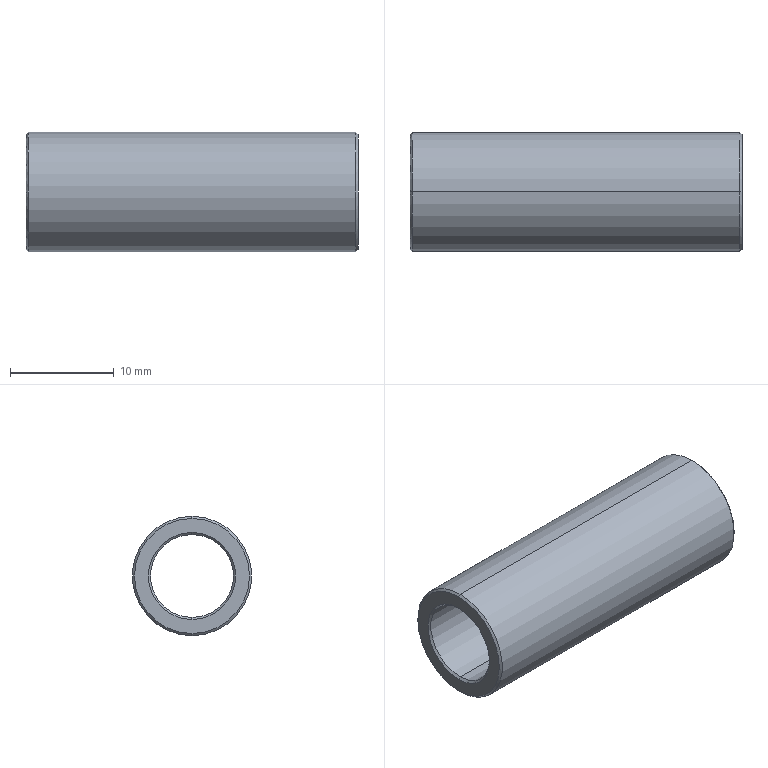Part | STEP file | FNCLSS-V8-D11.5-L32.0 | 1 solid | 14 faces | box 32 x 11.5 x 11.5 mm | volume 1713 mm3 | cone 8 | cylinder 4 | plane 2 | commonest cylinder face diameters 8 x2 11.5 x2
STEP:
#1=CARTESIAN_POINT('',(0.,0.,0.));
#2=DIRECTION('',(0.,0.,1.));
#3=DIRECTION('',(1.,0.,0.));
#4=AXIS2_PLACEMENT_3D('',#1,#2,#3);
#5=CARTESIAN_POINT('',(32.,0.,-5.55));
#6=VERTEX_POINT('',#5);
#7=CARTESIAN_POINT('',(32.,0.,5.55));
#8=VERTEX_POINT('',#7);
#9=CARTESIAN_POINT('',(32.,0.,0.));
#10=DIRECTION('',(1.,0.,0.));
#11=DIRECTION('',(0.,0.,1.));
#12=AXIS2_PLACEMENT_3D('',#9,#10,#11);
#13=CIRCLE('',#12,5.55);
#14=CARTESIAN_POINT('',(31.8,0.,0.));
#15=DIRECTION('',(-1.,0.,0.));
#16=DIRECTION('',(0.,0.,1.));
#17=AXIS2_PLACEMENT_3D('',#14,#15,#16);
#18=CONICAL_SURFACE('',#17,5.75,0.7854);
#19=CARTESIAN_POINT('',(6.283,-0.2));
#20=DIRECTION('',(-1.,0.));
#21=VECTOR('',#20,1.);
#22=LINE('',#19,#21);
#23=(GEOMETRIC_REPRESENTATION_CONTEXT(2)PARAMETRIC_REPRESENTATION_CONTEXT()REPRESENTATION_CONTEXT('',''));
#24=DEFINITIONAL_REPRESENTATION('',(#22),#23);
#25=PCURVE('',#18,#24);
#26=CARTESIAN_POINT('',(32.,4.,0.));
#27=DIRECTION('',(-1.,0.,0.));
#28=DIRECTION('',(0.,0.,1.));
#29=AXIS2_PLACEMENT_3D('',#26,#27,#28);
#30=PLANE('',#29);
#31=CARTESIAN_POINT('',(5.55,-4.));
#32=CARTESIAN_POINT('',(5.55,-13.613));
#33=CARTESIAN_POINT('',(-2.775,-8.806));
#34=CARTESIAN_POINT('',(-11.1,-4.));
#35=CARTESIAN_POINT('',(-2.775,0.8064));
#36=CARTESIAN_POINT('',(5.55,5.613));
#37=CARTESIAN_POINT('',(5.55,-4.));
#38=(BOUNDED_CURVE()B_SPLINE_CURVE(2,(#31,#32,#33,#34,#35,#36,#37),.UNSPECIFIED.,.T.,.F.)B_SPLINE_CURVE_WITH_KNOTS((1,2,2,2,2,1),(-2.094,0.,2.094,4.189,6.283,8.378),.UNSPECIFIED.)CURVE()GEOMETRIC_REPRESENTATION_ITEM()RATIONAL_B_SPLINE_CURVE((1.,0.5,1.,0.5,1.,0.5,1.))REPRESENTATION_ITEM(''));
#39=(GEOMETRIC_REPRESENTATION_CONTEXT(2)PARAMETRIC_REPRESENTATION_CONTEXT()REPRESENTATION_CONTEXT('',''));
#40=DEFINITIONAL_REPRESENTATION('',(#38),#39);
#41=PCURVE('',#30,#40);
#42=SURFACE_CURVE('',#13,(#25,#41),.PCURVE_S1.);
#43=EDGE_CURVE('',#6,#8,#42,.T.);
#44=ORIENTED_EDGE('',*,*,#43,.F.);
#45=CARTESIAN_POINT('',(31.8,0.,-5.75));
#46=VERTEX_POINT('',#45);
#47=CARTESIAN_POINT('',(31.8,0.,-5.75));
#48=DIRECTION('',(-0.7071,0.,-0.7071));
#49=VECTOR('',#48,1.);
#50=LINE('',#47,#49);
#51=CARTESIAN_POINT('',(3.142,0.));
#52=DIRECTION('',(0.,1.));
#53=VECTOR('',#52,1.);
#54=LINE('',#51,#53);
#55=(GEOMETRIC_REPRESENTATION_CONTEXT(2)PARAMETRIC_REPRESENTATION_CONTEXT()REPRESENTATION_CONTEXT('',''));
#56=DEFINITIONAL_REPRESENTATION('',(#54),#55);
#57=PCURVE('',#18,#56);
#58=CARTESIAN_POINT('',(31.8,0.,0.));
#59=DIRECTION('',(-1.,0.,0.));
#60=DIRECTION('',(0.,0.,1.));
#61=AXIS2_PLACEMENT_3D('',#58,#59,#60);
#62=CONICAL_SURFACE('',#61,5.75,0.7854);
#63=CARTESIAN_POINT('',(3.142,0.));
#64=DIRECTION('',(0.,1.));
#65=VECTOR('',#64,1.);
#66=LINE('',#63,#65);
#67=(GEOMETRIC_REPRESENTATION_CONTEXT(2)PARAMETRIC_REPRESENTATION_CONTEXT()REPRESENTATION_CONTEXT('',''));
#68=DEFINITIONAL_REPRESENTATION('',(#66),#67);
#69=PCURVE('',#62,#68);
#70=SURFACE_CURVE('',#50,(#57,#69),.PCURVE_S1.);
#71=EDGE_CURVE('',#6,#46,#70,.T.);
#72=ORIENTED_EDGE('',*,*,#71,.T.);
#73=CARTESIAN_POINT('',(31.8,0.,5.75));
#74=VERTEX_POINT('',#73);
#75=CARTESIAN_POINT('',(31.8,0.,0.));
#76=DIRECTION('',(-1.,0.,0.));
#77=DIRECTION('',(0.,0.,1.));
#78=AXIS2_PLACEMENT_3D('',#75,#76,#77);
#79=CIRCLE('',#78,5.75);
#80=CARTESIAN_POINT('',(0.,0.));
#81=DIRECTION('',(1.,0.));
#82=VECTOR('',#81,1.);
#83=LINE('',#80,#82);
#84=(GEOMETRIC_REPRESENTATION_CONTEXT(2)PARAMETRIC_REPRESENTATION_CONTEXT()REPRESENTATION_CONTEXT('',''));
#85=DEFINITIONAL_REPRESENTATION('',(#83),#84);
#86=PCURVE('',#18,#85);
#87=CARTESIAN_POINT('',(0.,0.,0.));
#88=DIRECTION('',(-1.,0.,0.));
#89=DIRECTION('',(0.,0.,1.));
#90=AXIS2_PLACEMENT_3D('',#87,#88,#89);
#91=CYLINDRICAL_SURFACE('',#90,5.75);
#92=CARTESIAN_POINT('',(0.,-31.8));
#93=DIRECTION('',(1.,0.));
#94=VECTOR('',#93,1.);
#95=LINE('',#92,#94);
#96=(GEOMETRIC_REPRESENTATION_CONTEXT(2)PARAMETRIC_REPRESENTATION_CONTEXT()REPRESENTATION_CONTEXT('',''));
#97=DEFINITIONAL_REPRESENTATION('',(#95),#96);
#98=PCURVE('',#91,#97);
#99=SURFACE_CURVE('',#79,(#86,#98),.PCURVE_S1.);
#100=EDGE_CURVE('',#74,#46,#99,.T.);
#101=ORIENTED_EDGE('',*,*,#100,.F.);
#102=CARTESIAN_POINT('',(31.8,0.,5.75));
#103=DIRECTION('',(-0.7071,0.,0.7071));
#104=VECTOR('',#103,1.);
#105=LINE('',#102,#104);
#106=CARTESIAN_POINT('',(0.,0.));
#107=DIRECTION('',(0.,1.));
#108=VECTOR('',#107,1.);
#109=LINE('',#106,#108);
#110=(GEOMETRIC_REPRESENTATION_CONTEXT(2)PARAMETRIC_REPRESENTATION_CONTEXT()REPRESENTATION_CONTEXT('',''));
#111=DEFINITIONAL_REPRESENTATION('',(#109),#110);
#112=PCURVE('',#18,#111);
#113=CARTESIAN_POINT('',(6.283,0.));
#114=DIRECTION('',(0.,1.));
#115=VECTOR('',#114,1.);
#116=LINE('',#113,#115);
#117=(GEOMETRIC_REPRESENTATION_CONTEXT(2)PARAMETRIC_REPRESENTATION_CONTEXT()REPRESENTATION_CONTEXT('',''));
#118=DEFINITIONAL_REPRESENTATION('',(#116),#117);
#119=PCURVE('',#62,#118);
#120=SURFACE_CURVE('',#105,(#112,#119),.PCURVE_S1.);
#121=EDGE_CURVE('',#8,#74,#120,.T.);
#122=ORIENTED_EDGE('',*,*,#121,.F.);
#123=EDGE_LOOP('',(#44,#72,#101,#122));
#124=FACE_BOUND('',#123,.T.);
#125=ADVANCED_FACE('',(#124),#18,.T.);
#126=CARTESIAN_POINT('',(31.8,0.,-4.));
#127=VERTEX_POINT('',#126);
#128=CARTESIAN_POINT('',(32.,0.,-4.2));
#129=VERTEX_POINT('',#128);
#130=CARTESIAN_POINT('',(32.,0.,-4.2));
#131=DIRECTION('',(0.7071,0.,-0.7071));
#132=VECTOR('',#131,1.);
#133=LINE('',#130,#132);
#134=CARTESIAN_POINT('',(32.,0.,0.));
#135=DIRECTION('',(1.,0.,0.));
#136=DIRECTION('',(0.,0.,-1.));
#137=AXIS2_PLACEMENT_3D('',#134,#135,#136);
#138=CONICAL_SURFACE('',#137,4.2,0.7854);
#139=CARTESIAN_POINT('',(6.283,0.));
#140=DIRECTION('',(0.,1.));
#141=VECTOR('',#140,1.);
#142=LINE('',#139,#141);
#143=(GEOMETRIC_REPRESENTATION_CONTEXT(2)PARAMETRIC_REPRESENTATION_CONTEXT()REPRESENTATION_CONTEXT('',''));
#144=DEFINITIONAL_REPRESENTATION('',(#142),#143);
#145=PCURVE('',#138,#144);
#146=CARTESIAN_POINT('',(32.,0.,0.));
#147=DIRECTION('',(1.,0.,0.));
#148=DIRECTION('',(0.,0.,-1.));
#149=AXIS2_PLACEMENT_3D('',#146,#147,#148);
#150=CONICAL_SURFACE('',#149,4.2,0.7854);
#151=CARTESIAN_POINT('',(0.,0.));
#152=DIRECTION('',(0.,1.));
#153=VECTOR('',#152,1.);
#154=LINE('',#151,#153);
#155=(GEOMETRIC_REPRESENTATION_CONTEXT(2)PARAMETRIC_REPRESENTATION_CONTEXT()REPRESENTATION_CONTEXT('',''));
#156=DEFINITIONAL_REPRESENTATION('',(#154),#155);
#157=PCURVE('',#150,#156);
#158=SURFACE_CURVE('',#133,(#145,#157),.PCURVE_S1.);
#159=EDGE_CURVE('',#127,#129,#158,.T.);
#160=ORIENTED_EDGE('',*,*,#159,.T.);
#161=CARTESIAN_POINT('',(32.,0.,4.2));
#162=VERTEX_POINT('',#161);
#163=CARTESIAN_POINT('',(32.,0.,0.));
#164=DIRECTION('',(-1.,0.,0.));
#165=DIRECTION('',(0.,0.,1.));
#166=AXIS2_PLACEMENT_3D('',#163,#164,#165);
#167=CIRCLE('',#166,4.2);
#168=CARTESIAN_POINT('',(9.425,0.));
#169=DIRECTION('',(-1.,0.));
#170=VECTOR('',#169,1.);
#171=LINE('',#168,#170);
#172=(GEOMETRIC_REPRESENTATION_CONTEXT(2)PARAMETRIC_REPRESENTATION_CONTEXT()REPRESENTATION_CONTEXT('',''));
#173=DEFINITIONAL_REPRESENTATION('',(#171),#172);
#174=PCURVE('',#138,#173);
#175=CARTESIAN_POINT('',(0.,-4.));
#176=DIRECTION('',(1.,0.));
#177=AXIS2_PLACEMENT_2D('',#175,#176);
#178=CIRCLE('',#177,4.2);
#179=(GEOMETRIC_REPRESENTATION_CONTEXT(2)PARAMETRIC_REPRESENTATION_CONTEXT()REPRESENTATION_CONTEXT('',''));
#180=DEFINITIONAL_REPRESENTATION('',(#178),#179);
#181=PCURVE('',#30,#180);
#182=SURFACE_CURVE('',#167,(#174,#181),.PCURVE_S1.);
#183=EDGE_CURVE('',#129,#162,#182,.T.);
#184=ORIENTED_EDGE('',*,*,#183,.T.);
#185=CARTESIAN_POINT('',(31.8,0.,4.));
#186=VERTEX_POINT('',#185);
#187=CARTESIAN_POINT('',(32.,0.,4.2));
#188=DIRECTION('',(0.7071,0.,0.7071));
#189=VECTOR('',#188,1.);
#190=LINE('',#187,#189);
#191=CARTESIAN_POINT('',(3.142,0.));
#192=DIRECTION('',(0.,1.));
#193=VECTOR('',#192,1.);
#194=LINE('',#191,#193);
#195=(GEOMETRIC_REPRESENTATION_CONTEXT(2)PARAMETRIC_REPRESENTATION_CONTEXT()REPRESENTATION_CONTEXT('',''));
#196=DEFINITIONAL_REPRESENTATION('',(#194),#195);
#197=PCURVE('',#138,#196);
#198=CARTESIAN_POINT('',(3.142,0.));
#199=DIRECTION('',(0.,1.));
#200=VECTOR('',#199,1.);
#201=LINE('',#198,#200);
#202=(GEOMETRIC_REPRESENTATION_CONTEXT(2)PARAMETRIC_REPRESENTATION_CONTEXT()REPRESENTATION_CONTEXT('',''));
#203=DEFINITIONAL_REPRESENTATION('',(#201),#202);
#204=PCURVE('',#150,#203);
#205=SURFACE_CURVE('',#190,(#197,#204),.PCURVE_S1.);
#206=EDGE_CURVE('',#186,#162,#205,.T.);
#207=ORIENTED_EDGE('',*,*,#206,.F.);
#208=CARTESIAN_POINT('',(31.8,0.,0.));
#209=DIRECTION('',(1.,0.,0.));
#210=DIRECTION('',(0.,0.,1.));
#211=AXIS2_PLACEMENT_3D('',#208,#209,#210);
#212=CIRCLE('',#211,4.);
#213=CARTESIAN_POINT('',(3.142,-0.2));
#214=DIRECTION('',(1.,0.));
#215=VECTOR('',#214,1.);
#216=LINE('',#213,#215);
#217=(GEOMETRIC_REPRESENTATION_CONTEXT(2)PARAMETRIC_REPRESENTATION_CONTEXT()REPRESENTATION_CONTEXT('',''));
#218=DEFINITIONAL_REPRESENTATION('',(#216),#217);
#219=PCURVE('',#138,#218);
#220=CARTESIAN_POINT('',(0.,0.,0.));
#221=DIRECTION('',(-1.,0.,0.));
#222=DIRECTION('',(0.,0.,1.));
#223=AXIS2_PLACEMENT_3D('',#220,#221,#222);
#224=CYLINDRICAL_SURFACE('',#223,4.);
#225=CARTESIAN_POINT('',(6.283,-31.8));
#226=DIRECTION('',(-1.,0.));
#227=VECTOR('',#226,1.);
#228=LINE('',#225,#227);
#229=(GEOMETRIC_REPRESENTATION_CONTEXT(2)PARAMETRIC_REPRESENTATION_CONTEXT()REPRESENTATION_CONTEXT('',''));
#230=DEFINITIONAL_REPRESENTATION('',(#228),#229);
#231=PCURVE('',#224,#230);
#232=SURFACE_CURVE('',#212,(#219,#231),.PCURVE_S1.);
#233=EDGE_CURVE('',#186,#127,#232,.T.);
#234=ORIENTED_EDGE('',*,*,#233,.T.);
#235=EDGE_LOOP('',(#160,#184,#207,#234));
#236=FACE_BOUND('',#235,.F.);
#237=ADVANCED_FACE('',(#236),#138,.F.);
#238=CARTESIAN_POINT('',(0.,0.,5.55));
#239=VERTEX_POINT('',#238);
#240=CARTESIAN_POINT('',(0.,0.,-5.55));
#241=VERTEX_POINT('',#240);
#242=CARTESIAN_POINT('',(0.,0.,0.));
#243=DIRECTION('',(-1.,0.,0.));
#244=DIRECTION('',(0.,0.,-1.));
#245=AXIS2_PLACEMENT_3D('',#242,#243,#244);
#246=CIRCLE('',#245,5.55);
#247=CARTESIAN_POINT('',(0.,0.,0.));
#248=DIRECTION('',(1.,0.,0.));
#249=DIRECTION('',(0.,0.,-1.));
#250=AXIS2_PLACEMENT_3D('',#247,#248,#249);
#251=CONICAL_SURFACE('',#250,5.55,0.7854);
#252=CARTESIAN_POINT('',(6.283,0.));
#253=DIRECTION('',(-1.,0.));
#254=VECTOR('',#253,1.);
#255=LINE('',#252,#254);
#256=(GEOMETRIC_REPRESENTATION_CONTEXT(2)PARAMETRIC_REPRESENTATION_CONTEXT()REPRESENTATION_CONTEXT('',''));
#257=DEFINITIONAL_REPRESENTATION('',(#255),#256);
#258=PCURVE('',#251,#257);
#259=CARTESIAN_POINT('',(0.,4.,0.));
#260=DIRECTION('',(1.,0.,0.));
#261=DIRECTION('',(0.,0.,-1.));
#262=AXIS2_PLACEMENT_3D('',#259,#260,#261);
#263=PLANE('',#262);
#264=CARTESIAN_POINT('',(5.55,-4.));
#265=CARTESIAN_POINT('',(5.55,-13.613));
#266=CARTESIAN_POINT('',(-2.775,-8.806));
#267=CARTESIAN_POINT('',(-11.1,-4.));
#268=CARTESIAN_POINT('',(-2.775,0.8064));
#269=CARTESIAN_POINT('',(5.55,5.613));
#270=CARTESIAN_POINT('',(5.55,-4.));
#271=(BOUNDED_CURVE()B_SPLINE_CURVE(2,(#264,#265,#266,#267,#268,#269,#270),.UNSPECIFIED.,.T.,.F.)B_SPLINE_CURVE_WITH_KNOTS((1,2,2,2,2,1),(-2.094,0.,2.094,4.189,6.283,8.378),.UNSPECIFIED.)CURVE()GEOMETRIC_REPRESENTATION_ITEM()RATIONAL_B_SPLINE_CURVE((1.,0.5,1.,0.5,1.,0.5,1.))REPRESENTATION_ITEM(''));
#272=(GEOMETRIC_REPRESENTATION_CONTEXT(2)PARAMETRIC_REPRESENTATION_CONTEXT()REPRESENTATION_CONTEXT('',''));
#273=DEFINITIONAL_REPRESENTATION('',(#271),#272);
#274=PCURVE('',#263,#273);
#275=SURFACE_CURVE('',#246,(#258,#274),.PCURVE_S1.);
#276=EDGE_CURVE('',#239,#241,#275,.T.);
#277=ORIENTED_EDGE('',*,*,#276,.F.);
#278=CARTESIAN_POINT('',(0.2,0.,5.75));
#279=VERTEX_POINT('',#278);
#280=CARTESIAN_POINT('',(0.,0.,5.55));
#281=DIRECTION('',(0.7071,0.,0.7071));
#282=VECTOR('',#281,1.);
#283=LINE('',#280,#282);
#284=CARTESIAN_POINT('',(3.142,0.));
#285=DIRECTION('',(0.,1.));
#286=VECTOR('',#285,1.);
#287=LINE('',#284,#286);
#288=(GEOMETRIC_REPRESENTATION_CONTEXT(2)PARAMETRIC_REPRESENTATION_CONTEXT()REPRESENTATION_CONTEXT('',''));
#289=DEFINITIONAL_REPRESENTATION('',(#287),#288);
#290=PCURVE('',#251,#289);
#291=CARTESIAN_POINT('',(0.,0.,0.));
#292=DIRECTION('',(1.,0.,0.));
#293=DIRECTION('',(0.,0.,-1.));
#294=AXIS2_PLACEMENT_3D('',#291,#292,#293);
#295=CONICAL_SURFACE('',#294,5.55,0.7854);
#296=CARTESIAN_POINT('',(3.142,0.));
#297=DIRECTION('',(0.,1.));
#298=VECTOR('',#297,1.);
#299=LINE('',#296,#298);
#300=(GEOMETRIC_REPRESENTATION_CONTEXT(2)PARAMETRIC_REPRESENTATION_CONTEXT()REPRESENTATION_CONTEXT('',''));
#301=DEFINITIONAL_REPRESENTATION('',(#299),#300);
#302=PCURVE('',#295,#301);
#303=SURFACE_CURVE('',#283,(#290,#302),.PCURVE_S1.);
#304=EDGE_CURVE('',#239,#279,#303,.T.);
#305=ORIENTED_EDGE('',*,*,#304,.T.);
#306=CARTESIAN_POINT('',(0.2,0.,-5.75));
#307=VERTEX_POINT('',#306);
#308=CARTESIAN_POINT('',(0.2,0.,0.));
#309=DIRECTION('',(1.,0.,0.));
#310=DIRECTION('',(0.,0.,-1.));
#311=AXIS2_PLACEMENT_3D('',#308,#309,#310);
#312=CIRCLE('',#311,5.75);
#313=CARTESIAN_POINT('',(0.,0.2));
#314=DIRECTION('',(1.,0.));
#315=VECTOR('',#314,1.);
#316=LINE('',#313,#315);
#317=(GEOMETRIC_REPRESENTATION_CONTEXT(2)PARAMETRIC_REPRESENTATION_CONTEXT()REPRESENTATION_CONTEXT('',''));
#318=DEFINITIONAL_REPRESENTATION('',(#316),#317);
#319=PCURVE('',#251,#318);
#320=CARTESIAN_POINT('',(3.142,-0.2));
#321=DIRECTION('',(-1.,0.));
#322=VECTOR('',#321,1.);
#323=LINE('',#320,#322);
#324=(GEOMETRIC_REPRESENTATION_CONTEXT(2)PARAMETRIC_REPRESENTATION_CONTEXT()REPRESENTATION_CONTEXT('',''));
#325=DEFINITIONAL_REPRESENTATION('',(#323),#324);
#326=PCURVE('',#91,#325);
#327=SURFACE_CURVE('',#312,(#319,#326),.PCURVE_S1.);
#328=EDGE_CURVE('',#307,#279,#327,.T.);
#329=ORIENTED_EDGE('',*,*,#328,.F.);
#330=CARTESIAN_POINT('',(0.,0.,-5.55));
#331=DIRECTION('',(0.7071,0.,-0.7071));
#332=VECTOR('',#331,1.);
#333=LINE('',#330,#332);
#334=CARTESIAN_POINT('',(0.,0.));
#335=DIRECTION('',(0.,1.));
#336=VECTOR('',#335,1.);
#337=LINE('',#334,#336);
#338=(GEOMETRIC_REPRESENTATION_CONTEXT(2)PARAMETRIC_REPRESENTATION_CONTEXT()REPRESENTATION_CONTEXT('',''));
#339=DEFINITIONAL_REPRESENTATION('',(#337),#338);
#340=PCURVE('',#251,#339);
#341=CARTESIAN_POINT('',(6.283,0.));
#342=DIRECTION('',(0.,1.));
#343=VECTOR('',#342,1.);
#344=LINE('',#341,#343);
#345=(GEOMETRIC_REPRESENTATION_CONTEXT(2)PARAMETRIC_REPRESENTATION_CONTEXT()REPRESENTATION_CONTEXT('',''));
#346=DEFINITIONAL_REPRESENTATION('',(#344),#345);
#347=PCURVE('',#295,#346);
#348=SURFACE_CURVE('',#333,(#340,#347),.PCURVE_S1.);
#349=EDGE_CURVE('',#241,#307,#348,.T.);
#350=ORIENTED_EDGE('',*,*,#349,.F.);
#351=EDGE_LOOP('',(#277,#305,#329,#350));
#352=FACE_BOUND('',#351,.T.);
#353=ADVANCED_FACE('',(#352),#251,.T.);
#354=CARTESIAN_POINT('',(0.2,0.,4.));
#355=VERTEX_POINT('',#354);
#356=CARTESIAN_POINT('',(0.,0.,4.2));
#357=VERTEX_POINT('',#356);
#358=CARTESIAN_POINT('',(0.2,0.,4.));
#359=DIRECTION('',(-0.7071,0.,0.7071));
#360=VECTOR('',#359,1.);
#361=LINE('',#358,#360);
#362=CARTESIAN_POINT('',(0.2,0.,0.));
#363=DIRECTION('',(-1.,0.,0.));
#364=DIRECTION('',(0.,0.,1.));
#365=AXIS2_PLACEMENT_3D('',#362,#363,#364);
#366=CONICAL_SURFACE('',#365,4.,0.7854);
#367=CARTESIAN_POINT('',(6.283,0.));
#368=DIRECTION('',(0.,1.));
#369=VECTOR('',#368,1.);
#370=LINE('',#367,#369);
#371=(GEOMETRIC_REPRESENTATION_CONTEXT(2)PARAMETRIC_REPRESENTATION_CONTEXT()REPRESENTATION_CONTEXT('',''));
#372=DEFINITIONAL_REPRESENTATION('',(#370),#371);
#373=PCURVE('',#366,#372);
#374=CARTESIAN_POINT('',(0.2,0.,0.));
#375=DIRECTION('',(-1.,0.,0.));
#376=DIRECTION('',(0.,0.,1.));
#377=AXIS2_PLACEMENT_3D('',#374,#375,#376);
#378=CONICAL_SURFACE('',#377,4.,0.7854);
#379=CARTESIAN_POINT('',(0.,0.));
#380=DIRECTION('',(0.,1.));
#381=VECTOR('',#380,1.);
#382=LINE('',#379,#381);
#383=(GEOMETRIC_REPRESENTATION_CONTEXT(2)PARAMETRIC_REPRESENTATION_CONTEXT()REPRESENTATION_CONTEXT('',''));
#384=DEFINITIONAL_REPRESENTATION('',(#382),#383);
#385=PCURVE('',#378,#384);
#386=SURFACE_CURVE('',#361,(#373,#385),.PCURVE_S1.);
#387=EDGE_CURVE('',#355,#357,#386,.T.);
#388=ORIENTED_EDGE('',*,*,#387,.T.);
#389=CARTESIAN_POINT('',(0.,0.,-4.2));
#390=VERTEX_POINT('',#389);
#391=CARTESIAN_POINT('',(0.,0.,0.));
#392=DIRECTION('',(1.,0.,0.));
#393=DIRECTION('',(0.,0.,-1.));
#394=AXIS2_PLACEMENT_3D('',#391,#392,#393);
#395=CIRCLE('',#394,4.2);
#396=CARTESIAN_POINT('',(9.425,0.2));
#397=DIRECTION('',(-1.,0.));
#398=VECTOR('',#397,1.);
#399=LINE('',#396,#398);
#400=(GEOMETRIC_REPRESENTATION_CONTEXT(2)PARAMETRIC_REPRESENTATION_CONTEXT()REPRESENTATION_CONTEXT('',''));
#401=DEFINITIONAL_REPRESENTATION('',(#399),#400);
#402=PCURVE('',#366,#401);
#403=CARTESIAN_POINT('',(0.,-4.));
#404=DIRECTION('',(1.,0.));
#405=AXIS2_PLACEMENT_2D('',#403,#404);
#406=CIRCLE('',#405,4.2);
#407=(GEOMETRIC_REPRESENTATION_CONTEXT(2)PARAMETRIC_REPRESENTATION_CONTEXT()REPRESENTATION_CONTEXT('',''));
#408=DEFINITIONAL_REPRESENTATION('',(#406),#407);
#409=PCURVE('',#263,#408);
#410=SURFACE_CURVE('',#395,(#402,#409),.PCURVE_S1.);
#411=EDGE_CURVE('',#357,#390,#410,.T.);
#412=ORIENTED_EDGE('',*,*,#411,.T.);
#413=CARTESIAN_POINT('',(0.2,0.,-4.));
#414=VERTEX_POINT('',#413);
#415=CARTESIAN_POINT('',(0.2,0.,-4.));
#416=DIRECTION('',(-0.7071,0.,-0.7071));
#417=VECTOR('',#416,1.);
#418=LINE('',#415,#417);
#419=CARTESIAN_POINT('',(3.142,0.));
#420=DIRECTION('',(0.,1.));
#421=VECTOR('',#420,1.);
#422=LINE('',#419,#421);
#423=(GEOMETRIC_REPRESENTATION_CONTEXT(2)PARAMETRIC_REPRESENTATION_CONTEXT()REPRESENTATION_CONTEXT('',''));
#424=DEFINITIONAL_REPRESENTATION('',(#422),#423);
#425=PCURVE('',#366,#424);
#426=CARTESIAN_POINT('',(3.142,0.));
#427=DIRECTION('',(0.,1.));
#428=VECTOR('',#427,1.);
#429=LINE('',#426,#428);
#430=(GEOMETRIC_REPRESENTATION_CONTEXT(2)PARAMETRIC_REPRESENTATION_CONTEXT()REPRESENTATION_CONTEXT('',''));
#431=DEFINITIONAL_REPRESENTATION('',(#429),#430);
#432=PCURVE('',#378,#431);
#433=SURFACE_CURVE('',#418,(#425,#432),.PCURVE_S1.);
#434=EDGE_CURVE('',#414,#390,#433,.T.);
#435=ORIENTED_EDGE('',*,*,#434,.F.);
#436=CARTESIAN_POINT('',(0.2,0.,0.));
#437=DIRECTION('',(-1.,0.,0.));
#438=DIRECTION('',(0.,0.,-1.));
#439=AXIS2_PLACEMENT_3D('',#436,#437,#438);
#440=CIRCLE('',#439,4.);
#441=CARTESIAN_POINT('',(3.142,0.));
#442=DIRECTION('',(1.,0.));
#443=VECTOR('',#442,1.);
#444=LINE('',#441,#443);
#445=(GEOMETRIC_REPRESENTATION_CONTEXT(2)PARAMETRIC_REPRESENTATION_CONTEXT()REPRESENTATION_CONTEXT('',''));
#446=DEFINITIONAL_REPRESENTATION('',(#444),#445);
#447=PCURVE('',#366,#446);
#448=CARTESIAN_POINT('',(3.142,-0.2));
#449=DIRECTION('',(1.,0.));
#450=VECTOR('',#449,1.);
#451=LINE('',#448,#450);
#452=(GEOMETRIC_REPRESENTATION_CONTEXT(2)PARAMETRIC_REPRESENTATION_CONTEXT()REPRESENTATION_CONTEXT('',''));
#453=DEFINITIONAL_REPRESENTATION('',(#451),#452);
#454=PCURVE('',#224,#453);
#455=SURFACE_CURVE('',#440,(#447,#454),.PCURVE_S1.);
#456=EDGE_CURVE('',#414,#355,#455,.T.);
#457=ORIENTED_EDGE('',*,*,#456,.T.);
#458=EDGE_LOOP('',(#388,#412,#435,#457));
#459=FACE_BOUND('',#458,.F.);
#460=ADVANCED_FACE('',(#459),#366,.F.);
#461=CARTESIAN_POINT('',(0.,0.,4.));
#462=DIRECTION('',(-1.,0.,0.));
#463=VECTOR('',#462,1.);
#464=LINE('',#461,#463);
#465=CARTESIAN_POINT('',(6.283,0.));
#466=DIRECTION('',(0.,1.));
#467=VECTOR('',#466,1.);
#468=LINE('',#465,#467);
#469=(GEOMETRIC_REPRESENTATION_CONTEXT(2)PARAMETRIC_REPRESENTATION_CONTEXT()REPRESENTATION_CONTEXT('',''));
#470=DEFINITIONAL_REPRESENTATION('',(#468),#469);
#471=PCURVE('',#224,#470);
#472=CARTESIAN_POINT('',(0.,0.,0.));
#473=DIRECTION('',(-1.,0.,0.));
#474=DIRECTION('',(0.,0.,1.));
#475=AXIS2_PLACEMENT_3D('',#472,#473,#474);
#476=CYLINDRICAL_SURFACE('',#475,4.);
#477=CARTESIAN_POINT('',(0.,0.));
#478=DIRECTION('',(0.,1.));
#479=VECTOR('',#478,1.);
#480=LINE('',#477,#479);
#481=(GEOMETRIC_REPRESENTATION_CONTEXT(2)PARAMETRIC_REPRESENTATION_CONTEXT()REPRESENTATION_CONTEXT('',''));
#482=DEFINITIONAL_REPRESENTATION('',(#480),#481);
#483=PCURVE('',#476,#482);
#484=SURFACE_CURVE('',#464,(#471,#483),.PCURVE_S1.);
#485=EDGE_CURVE('',#186,#355,#484,.T.);
#486=ORIENTED_EDGE('',*,*,#485,.T.);
#487=ORIENTED_EDGE('',*,*,#456,.F.);
#488=CARTESIAN_POINT('',(0.,0.,-4.));
#489=DIRECTION('',(-1.,0.,0.));
#490=VECTOR('',#489,1.);
#491=LINE('',#488,#490);
#492=CARTESIAN_POINT('',(3.142,0.));
#493=DIRECTION('',(0.,1.));
#494=VECTOR('',#493,1.);
#495=LINE('',#492,#494);
#496=(GEOMETRIC_REPRESENTATION_CONTEXT(2)PARAMETRIC_REPRESENTATION_CONTEXT()REPRESENTATION_CONTEXT('',''));
#497=DEFINITIONAL_REPRESENTATION('',(#495),#496);
#498=PCURVE('',#224,#497);
#499=CARTESIAN_POINT('',(3.142,0.));
#500=DIRECTION('',(0.,1.));
#501=VECTOR('',#500,1.);
#502=LINE('',#499,#501);
#503=(GEOMETRIC_REPRESENTATION_CONTEXT(2)PARAMETRIC_REPRESENTATION_CONTEXT()REPRESENTATION_CONTEXT('',''));
#504=DEFINITIONAL_REPRESENTATION('',(#502),#503);
#505=PCURVE('',#476,#504);
#506=SURFACE_CURVE('',#491,(#498,#505),.PCURVE_S1.);
#507=EDGE_CURVE('',#127,#414,#506,.T.);
#508=ORIENTED_EDGE('',*,*,#507,.F.);
#509=ORIENTED_EDGE('',*,*,#233,.F.);
#510=EDGE_LOOP('',(#486,#487,#508,#509));
#511=FACE_BOUND('',#510,.F.);
#512=ADVANCED_FACE('',(#511),#224,.F.);
#513=ORIENTED_EDGE('',*,*,#100,.T.);
#514=CARTESIAN_POINT('',(0.,0.,-5.75));
#515=DIRECTION('',(-1.,0.,0.));
#516=VECTOR('',#515,1.);
#517=LINE('',#514,#516);
#518=CARTESIAN_POINT('',(3.142,0.));
#519=DIRECTION('',(0.,1.));
#520=VECTOR('',#519,1.);
#521=LINE('',#518,#520);
#522=(GEOMETRIC_REPRESENTATION_CONTEXT(2)PARAMETRIC_REPRESENTATION_CONTEXT()REPRESENTATION_CONTEXT('',''));
#523=DEFINITIONAL_REPRESENTATION('',(#521),#522);
#524=PCURVE('',#91,#523);
#525=CARTESIAN_POINT('',(0.,0.,0.));
#526=DIRECTION('',(-1.,0.,0.));
#527=DIRECTION('',(0.,0.,1.));
#528=AXIS2_PLACEMENT_3D('',#525,#526,#527);
#529=CYLINDRICAL_SURFACE('',#528,5.75);
#530=CARTESIAN_POINT('',(3.142,0.));
#531=DIRECTION('',(0.,1.));
#532=VECTOR('',#531,1.);
#533=LINE('',#530,#532);
#534=(GEOMETRIC_REPRESENTATION_CONTEXT(2)PARAMETRIC_REPRESENTATION_CONTEXT()REPRESENTATION_CONTEXT('',''));
#535=DEFINITIONAL_REPRESENTATION('',(#533),#534);
#536=PCURVE('',#529,#535);
#537=SURFACE_CURVE('',#517,(#524,#536),.PCURVE_S1.);
#538=EDGE_CURVE('',#46,#307,#537,.T.);
#539=ORIENTED_EDGE('',*,*,#538,.T.);
#540=ORIENTED_EDGE('',*,*,#328,.T.);
#541=CARTESIAN_POINT('',(0.,0.,5.75));
#542=DIRECTION('',(-1.,0.,0.));
#543=VECTOR('',#542,1.);
#544=LINE('',#541,#543);
#545=CARTESIAN_POINT('',(0.,0.));
#546=DIRECTION('',(0.,1.));
#547=VECTOR('',#546,1.);
#548=LINE('',#545,#547);
#549=(GEOMETRIC_REPRESENTATION_CONTEXT(2)PARAMETRIC_REPRESENTATION_CONTEXT()REPRESENTATION_CONTEXT('',''));
#550=DEFINITIONAL_REPRESENTATION('',(#548),#549);
#551=PCURVE('',#91,#550);
#552=CARTESIAN_POINT('',(6.283,0.));
#553=DIRECTION('',(0.,1.));
#554=VECTOR('',#553,1.);
#555=LINE('',#552,#554);
#556=(GEOMETRIC_REPRESENTATION_CONTEXT(2)PARAMETRIC_REPRESENTATION_CONTEXT()REPRESENTATION_CONTEXT('',''));
#557=DEFINITIONAL_REPRESENTATION('',(#555),#556);
#558=PCURVE('',#529,#557);
#559=SURFACE_CURVE('',#544,(#551,#558),.PCURVE_S1.);
#560=EDGE_CURVE('',#74,#279,#559,.T.);
#561=ORIENTED_EDGE('',*,*,#560,.F.);
#562=EDGE_LOOP('',(#513,#539,#540,#561));
#563=FACE_BOUND('',#562,.T.);
#564=ADVANCED_FACE('',(#563),#91,.T.);
#565=ORIENTED_EDGE('',*,*,#411,.T.);
#566=CARTESIAN_POINT('',(0.,0.,0.));
#567=DIRECTION('',(1.,0.,0.));
#568=DIRECTION('',(0.,0.,-1.));
#569=AXIS2_PLACEMENT_3D('',#566,#567,#568);
#570=CIRCLE('',#569,4.2);
#571=CARTESIAN_POINT('',(0.,-4.));
#572=DIRECTION('',(1.,0.));
#573=AXIS2_PLACEMENT_2D('',#571,#572);
#574=CIRCLE('',#573,4.2);
#575=(GEOMETRIC_REPRESENTATION_CONTEXT(2)PARAMETRIC_REPRESENTATION_CONTEXT()REPRESENTATION_CONTEXT('',''));
#576=DEFINITIONAL_REPRESENTATION('',(#574),#575);
#577=PCURVE('',#263,#576);
#578=CARTESIAN_POINT('',(3.142,0.2));
#579=DIRECTION('',(-1.,0.));
#580=VECTOR('',#579,1.);
#581=LINE('',#578,#580);
#582=(GEOMETRIC_REPRESENTATION_CONTEXT(2)PARAMETRIC_REPRESENTATION_CONTEXT()REPRESENTATION_CONTEXT('',''));
#583=DEFINITIONAL_REPRESENTATION('',(#581),#582);
#584=PCURVE('',#378,#583);
#585=SURFACE_CURVE('',#570,(#577,#584),.PCURVE_S1.);
#586=EDGE_CURVE('',#390,#357,#585,.T.);
#587=ORIENTED_EDGE('',*,*,#586,.T.);
#588=EDGE_LOOP('',(#565,#587));
#589=FACE_BOUND('',#588,.T.);
#590=CARTESIAN_POINT('',(0.,0.,0.));
#591=DIRECTION('',(-1.,0.,0.));
#592=DIRECTION('',(0.,0.,-1.));
#593=AXIS2_PLACEMENT_3D('',#590,#591,#592);
#594=CIRCLE('',#593,5.55);
#595=CARTESIAN_POINT('',(5.55,-4.));
#596=CARTESIAN_POINT('',(5.55,-13.613));
#597=CARTESIAN_POINT('',(-2.775,-8.806));
#598=CARTESIAN_POINT('',(-11.1,-4.));
#599=CARTESIAN_POINT('',(-2.775,0.8064));
#600=CARTESIAN_POINT('',(5.55,5.613));
#601=CARTESIAN_POINT('',(5.55,-4.));
#602=(BOUNDED_CURVE()B_SPLINE_CURVE(2,(#595,#596,#597,#598,#599,#600,#601),.UNSPECIFIED.,.T.,.F.)B_SPLINE_CURVE_WITH_KNOTS((1,2,2,2,2,1),(-2.094,0.,2.094,4.189,6.283,8.378),.UNSPECIFIED.)CURVE()GEOMETRIC_REPRESENTATION_ITEM()RATIONAL_B_SPLINE_CURVE((1.,0.5,1.,0.5,1.,0.5,1.))REPRESENTATION_ITEM(''));
#603=(GEOMETRIC_REPRESENTATION_CONTEXT(2)PARAMETRIC_REPRESENTATION_CONTEXT()REPRESENTATION_CONTEXT('',''));
#604=DEFINITIONAL_REPRESENTATION('',(#602),#603);
#605=PCURVE('',#263,#604);
#606=CARTESIAN_POINT('',(6.283,0.));
#607=DIRECTION('',(-1.,0.));
#608=VECTOR('',#607,1.);
#609=LINE('',#606,#608);
#610=(GEOMETRIC_REPRESENTATION_CONTEXT(2)PARAMETRIC_REPRESENTATION_CONTEXT()REPRESENTATION_CONTEXT('',''));
#611=DEFINITIONAL_REPRESENTATION('',(#609),#610);
#612=PCURVE('',#295,#611);
#613=SURFACE_CURVE('',#594,(#605,#612),.PCURVE_S1.);
#614=EDGE_CURVE('',#241,#239,#613,.T.);
#615=ORIENTED_EDGE('',*,*,#614,.T.);
#616=ORIENTED_EDGE('',*,*,#276,.T.);
#617=EDGE_LOOP('',(#615,#616));
#618=FACE_BOUND('',#617,.T.);
#619=ADVANCED_FACE('',(#589,#618),#263,.F.);
#620=ORIENTED_EDGE('',*,*,#538,.F.);
#621=CARTESIAN_POINT('',(31.8,0.,0.));
#622=DIRECTION('',(-1.,0.,0.));
#623=DIRECTION('',(0.,0.,1.));
#624=AXIS2_PLACEMENT_3D('',#621,#622,#623);
#625=CIRCLE('',#624,5.75);
#626=CARTESIAN_POINT('',(0.,-31.8));
#627=DIRECTION('',(1.,0.));
#628=VECTOR('',#627,1.);
#629=LINE('',#626,#628);
#630=(GEOMETRIC_REPRESENTATION_CONTEXT(2)PARAMETRIC_REPRESENTATION_CONTEXT()REPRESENTATION_CONTEXT('',''));
#631=DEFINITIONAL_REPRESENTATION('',(#629),#630);
#632=PCURVE('',#529,#631);
#633=CARTESIAN_POINT('',(0.,0.));
#634=DIRECTION('',(1.,0.));
#635=VECTOR('',#634,1.);
#636=LINE('',#633,#635);
#637=(GEOMETRIC_REPRESENTATION_CONTEXT(2)PARAMETRIC_REPRESENTATION_CONTEXT()REPRESENTATION_CONTEXT('',''));
#638=DEFINITIONAL_REPRESENTATION('',(#636),#637);
#639=PCURVE('',#62,#638);
#640=SURFACE_CURVE('',#625,(#632,#639),.PCURVE_S1.);
#641=EDGE_CURVE('',#46,#74,#640,.T.);
#642=ORIENTED_EDGE('',*,*,#641,.T.);
#643=ORIENTED_EDGE('',*,*,#560,.T.);
#644=CARTESIAN_POINT('',(0.2,0.,0.));
#645=DIRECTION('',(1.,0.,0.));
#646=DIRECTION('',(0.,0.,-1.));
#647=AXIS2_PLACEMENT_3D('',#644,#645,#646);
#648=CIRCLE('',#647,5.75);
#649=CARTESIAN_POINT('',(9.425,-0.2));
#650=DIRECTION('',(-1.,0.));
#651=VECTOR('',#650,1.);
#652=LINE('',#649,#651);
#653=(GEOMETRIC_REPRESENTATION_CONTEXT(2)PARAMETRIC_REPRESENTATION_CONTEXT()REPRESENTATION_CONTEXT('',''));
#654=DEFINITIONAL_REPRESENTATION('',(#652),#653);
#655=PCURVE('',#529,#654);
#656=CARTESIAN_POINT('',(0.,0.2));
#657=DIRECTION('',(1.,0.));
#658=VECTOR('',#657,1.);
#659=LINE('',#656,#658);
#660=(GEOMETRIC_REPRESENTATION_CONTEXT(2)PARAMETRIC_REPRESENTATION_CONTEXT()REPRESENTATION_CONTEXT('',''));
#661=DEFINITIONAL_REPRESENTATION('',(#659),#660);
#662=PCURVE('',#295,#661);
#663=SURFACE_CURVE('',#648,(#655,#662),.PCURVE_S1.);
#664=EDGE_CURVE('',#279,#307,#663,.T.);
#665=ORIENTED_EDGE('',*,*,#664,.T.);
#666=EDGE_LOOP('',(#620,#642,#643,#665));
#667=FACE_BOUND('',#666,.T.);
#668=ADVANCED_FACE('',(#667),#529,.T.);
#669=ORIENTED_EDGE('',*,*,#183,.T.);
#670=CARTESIAN_POINT('',(32.,0.,0.));
#671=DIRECTION('',(-1.,0.,0.));
#672=DIRECTION('',(0.,0.,1.));
#673=AXIS2_PLACEMENT_3D('',#670,#671,#672);
#674=CIRCLE('',#673,4.2);
#675=CARTESIAN_POINT('',(0.,-4.));
#676=DIRECTION('',(1.,0.));
#677=AXIS2_PLACEMENT_2D('',#675,#676);
#678=CIRCLE('',#677,4.2);
#679=(GEOMETRIC_REPRESENTATION_CONTEXT(2)PARAMETRIC_REPRESENTATION_CONTEXT()REPRESENTATION_CONTEXT('',''));
#680=DEFINITIONAL_REPRESENTATION('',(#678),#679);
#681=PCURVE('',#30,#680);
#682=CARTESIAN_POINT('',(3.142,0.));
#683=DIRECTION('',(-1.,0.));
#684=VECTOR('',#683,1.);
#685=LINE('',#682,#684);
#686=(GEOMETRIC_REPRESENTATION_CONTEXT(2)PARAMETRIC_REPRESENTATION_CONTEXT()REPRESENTATION_CONTEXT('',''));
#687=DEFINITIONAL_REPRESENTATION('',(#685),#686);
#688=PCURVE('',#150,#687);
#689=SURFACE_CURVE('',#674,(#681,#688),.PCURVE_S1.);
#690=EDGE_CURVE('',#162,#129,#689,.T.);
#691=ORIENTED_EDGE('',*,*,#690,.T.);
#692=EDGE_LOOP('',(#669,#691));
#693=FACE_BOUND('',#692,.T.);
#694=CARTESIAN_POINT('',(32.,0.,0.));
#695=DIRECTION('',(1.,0.,0.));
#696=DIRECTION('',(0.,0.,1.));
#697=AXIS2_PLACEMENT_3D('',#694,#695,#696);
#698=CIRCLE('',#697,5.55);
#699=CARTESIAN_POINT('',(5.55,-4.));
#700=CARTESIAN_POINT('',(5.55,-13.613));
#701=CARTESIAN_POINT('',(-2.775,-8.806));
#702=CARTESIAN_POINT('',(-11.1,-4.));
#703=CARTESIAN_POINT('',(-2.775,0.8064));
#704=CARTESIAN_POINT('',(5.55,5.613));
#705=CARTESIAN_POINT('',(5.55,-4.));
#706=(BOUNDED_CURVE()B_SPLINE_CURVE(2,(#699,#700,#701,#702,#703,#704,#705),.UNSPECIFIED.,.T.,.F.)B_SPLINE_CURVE_WITH_KNOTS((1,2,2,2,2,1),(-2.094,0.,2.094,4.189,6.283,8.378),.UNSPECIFIED.)CURVE()GEOMETRIC_REPRESENTATION_ITEM()RATIONAL_B_SPLINE_CURVE((1.,0.5,1.,0.5,1.,0.5,1.))REPRESENTATION_ITEM(''));
#707=(GEOMETRIC_REPRESENTATION_CONTEXT(2)PARAMETRIC_REPRESENTATION_CONTEXT()REPRESENTATION_CONTEXT('',''));
#708=DEFINITIONAL_REPRESENTATION('',(#706),#707);
#709=PCURVE('',#30,#708);
#710=CARTESIAN_POINT('',(6.283,-0.2));
#711=DIRECTION('',(-1.,0.));
#712=VECTOR('',#711,1.);
#713=LINE('',#710,#712);
#714=(GEOMETRIC_REPRESENTATION_CONTEXT(2)PARAMETRIC_REPRESENTATION_CONTEXT()REPRESENTATION_CONTEXT('',''));
#715=DEFINITIONAL_REPRESENTATION('',(#713),#714);
#716=PCURVE('',#62,#715);
#717=SURFACE_CURVE('',#698,(#709,#716),.PCURVE_S1.);
#718=EDGE_CURVE('',#8,#6,#717,.T.);
#719=ORIENTED_EDGE('',*,*,#718,.T.);
#720=ORIENTED_EDGE('',*,*,#43,.T.);
#721=EDGE_LOOP('',(#719,#720));
#722=FACE_BOUND('',#721,.T.);
#723=ADVANCED_FACE('',(#693,#722),#30,.F.);
#724=CARTESIAN_POINT('',(0.2,0.,0.));
#725=DIRECTION('',(-1.,0.,0.));
#726=DIRECTION('',(0.,0.,-1.));
#727=AXIS2_PLACEMENT_3D('',#724,#725,#726);
#728=CIRCLE('',#727,4.);
#729=CARTESIAN_POINT('',(-3.142,-0.2));
#730=DIRECTION('',(1.,0.));
#731=VECTOR('',#730,1.);
#732=LINE('',#729,#731);
#733=(GEOMETRIC_REPRESENTATION_CONTEXT(2)PARAMETRIC_REPRESENTATION_CONTEXT()REPRESENTATION_CONTEXT('',''));
#734=DEFINITIONAL_REPRESENTATION('',(#732),#733);
#735=PCURVE('',#476,#734);
#736=CARTESIAN_POINT('',(-3.142,0.));
#737=DIRECTION('',(1.,0.));
#738=VECTOR('',#737,1.);
#739=LINE('',#736,#738);
#740=(GEOMETRIC_REPRESENTATION_CONTEXT(2)PARAMETRIC_REPRESENTATION_CONTEXT()REPRESENTATION_CONTEXT('',''));
#741=DEFINITIONAL_REPRESENTATION('',(#739),#740);
#742=PCURVE('',#378,#741);
#743=SURFACE_CURVE('',#728,(#735,#742),.PCURVE_S1.);
#744=EDGE_CURVE('',#355,#414,#743,.T.);
#745=ORIENTED_EDGE('',*,*,#744,.F.);
#746=ORIENTED_EDGE('',*,*,#485,.F.);
#747=CARTESIAN_POINT('',(31.8,0.,0.));
#748=DIRECTION('',(1.,0.,0.));
#749=DIRECTION('',(0.,0.,1.));
#750=AXIS2_PLACEMENT_3D('',#747,#748,#749);
#751=CIRCLE('',#750,4.);
#752=CARTESIAN_POINT('',(6.283,-31.8));
#753=DIRECTION('',(-1.,0.));
#754=VECTOR('',#753,1.);
#755=LINE('',#752,#754);
#756=(GEOMETRIC_REPRESENTATION_CONTEXT(2)PARAMETRIC_REPRESENTATION_CONTEXT()REPRESENTATION_CONTEXT('',''));
#757=DEFINITIONAL_REPRESENTATION('',(#755),#756);
#758=PCURVE('',#476,#757);
#759=CARTESIAN_POINT('',(-3.142,-0.2));
#760=DIRECTION('',(1.,0.));
#761=VECTOR('',#760,1.);
#762=LINE('',#759,#761);
#763=(GEOMETRIC_REPRESENTATION_CONTEXT(2)PARAMETRIC_REPRESENTATION_CONTEXT()REPRESENTATION_CONTEXT('',''));
#764=DEFINITIONAL_REPRESENTATION('',(#762),#763);
#765=PCURVE('',#150,#764);
#766=SURFACE_CURVE('',#751,(#758,#765),.PCURVE_S1.);
#767=EDGE_CURVE('',#127,#186,#766,.T.);
#768=ORIENTED_EDGE('',*,*,#767,.F.);
#769=ORIENTED_EDGE('',*,*,#507,.T.);
#770=EDGE_LOOP('',(#745,#746,#768,#769));
#771=FACE_BOUND('',#770,.F.);
#772=ADVANCED_FACE('',(#771),#476,.F.);
#773=ORIENTED_EDGE('',*,*,#586,.T.);
#774=ORIENTED_EDGE('',*,*,#387,.F.);
#775=ORIENTED_EDGE('',*,*,#744,.T.);
#776=ORIENTED_EDGE('',*,*,#434,.T.);
#777=EDGE_LOOP('',(#773,#774,#775,#776));
#778=FACE_BOUND('',#777,.F.);
#779=ADVANCED_FACE('',(#778),#378,.F.);
#780=ORIENTED_EDGE('',*,*,#304,.F.);
#781=ORIENTED_EDGE('',*,*,#614,.F.);
#782=ORIENTED_EDGE('',*,*,#349,.T.);
#783=ORIENTED_EDGE('',*,*,#664,.F.);
#784=EDGE_LOOP('',(#780,#781,#782,#783));
#785=FACE_BOUND('',#784,.T.);
#786=ADVANCED_FACE('',(#785),#295,.T.);
#787=ORIENTED_EDGE('',*,*,#690,.T.);
#788=ORIENTED_EDGE('',*,*,#159,.F.);
#789=ORIENTED_EDGE('',*,*,#767,.T.);
#790=ORIENTED_EDGE('',*,*,#206,.T.);
#791=EDGE_LOOP('',(#787,#788,#789,#790));
#792=FACE_BOUND('',#791,.F.);
#793=ADVANCED_FACE('',(#792),#150,.F.);
#794=ORIENTED_EDGE('',*,*,#71,.F.);
#795=ORIENTED_EDGE('',*,*,#718,.F.);
#796=ORIENTED_EDGE('',*,*,#121,.T.);
#797=ORIENTED_EDGE('',*,*,#641,.F.);
#798=EDGE_LOOP('',(#794,#795,#796,#797));
#799=FACE_BOUND('',#798,.T.);
#800=ADVANCED_FACE('',(#799),#62,.T.);
#801=CLOSED_SHELL('',(#125,#237,#353,#460,#512,#564,#619,#668,#723,#772,#779,#786,#793,#800));
#802=MANIFOLD_SOLID_BREP('',#801);
#803=(LENGTH_UNIT()NAMED_UNIT(*)SI_UNIT(.MILLI.,.METRE.));
#804=UNCERTAINTY_MEASURE_WITH_UNIT(LENGTH_MEASURE(0.0000001),#803,'','');
#805=(NAMED_UNIT(*)PLANE_ANGLE_UNIT()SI_UNIT($,.RADIAN.));
#806=(NAMED_UNIT(*)SI_UNIT($,.STERADIAN.)SOLID_ANGLE_UNIT());
#807=(GEOMETRIC_REPRESENTATION_CONTEXT(3)GLOBAL_UNCERTAINTY_ASSIGNED_CONTEXT((#804))GLOBAL_UNIT_ASSIGNED_CONTEXT((#803,#805,#806))REPRESENTATION_CONTEXT('',''));
#808=ADVANCED_BREP_SHAPE_REPRESENTATION('',(#4,#802),#807);